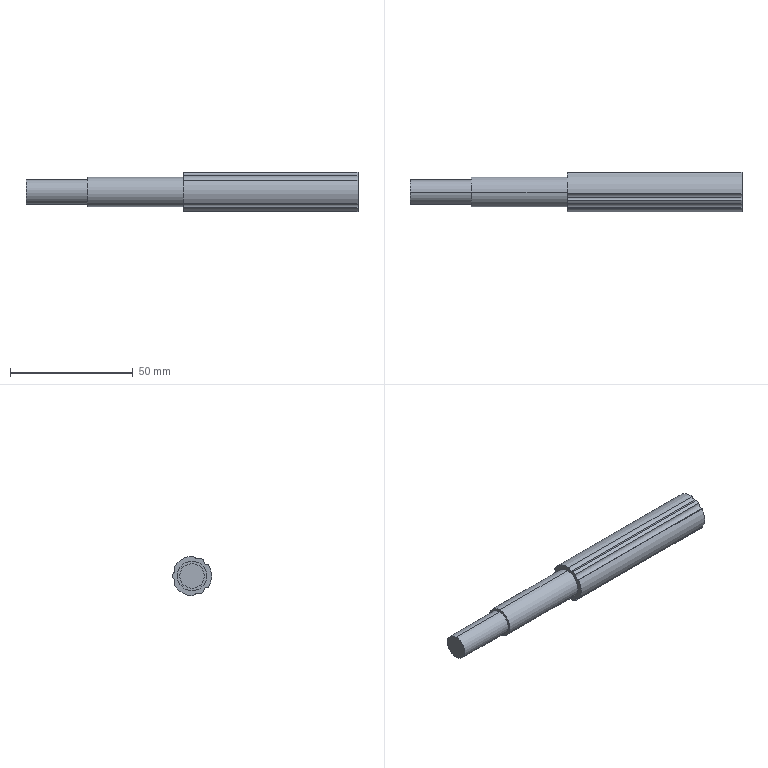Part | STEP file | SceondHI_LTR 16A150 LTRA Shaft_Default | 1 solid | 23 faces | box 135 x 16 x 16 mm | volume 20071 mm3 | cylinder 19 | plane 4 | commonest cylinder face diameters 3.3 x8 16 x7 10 x2 12 x2